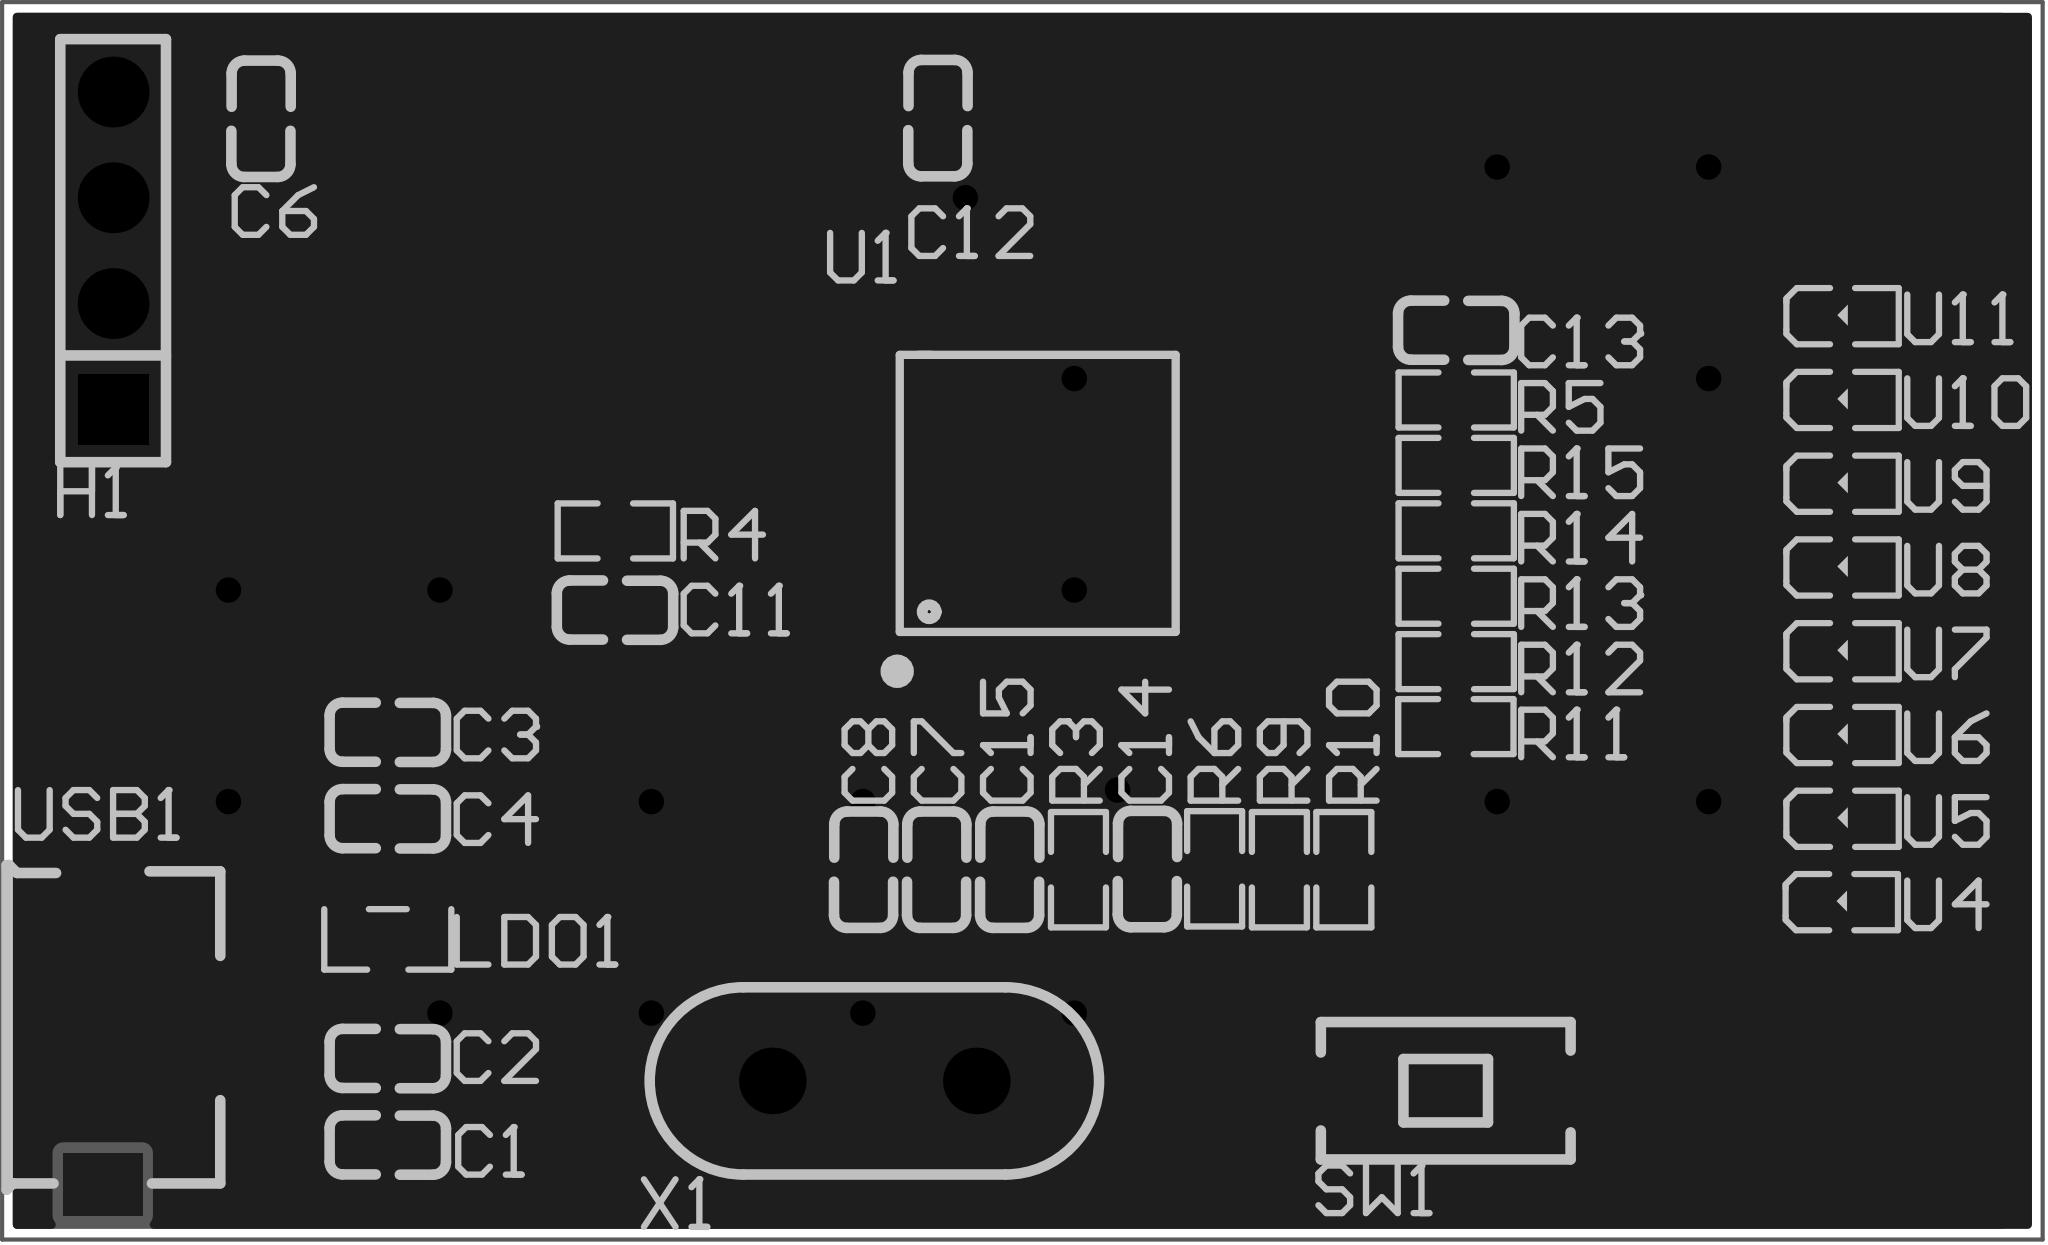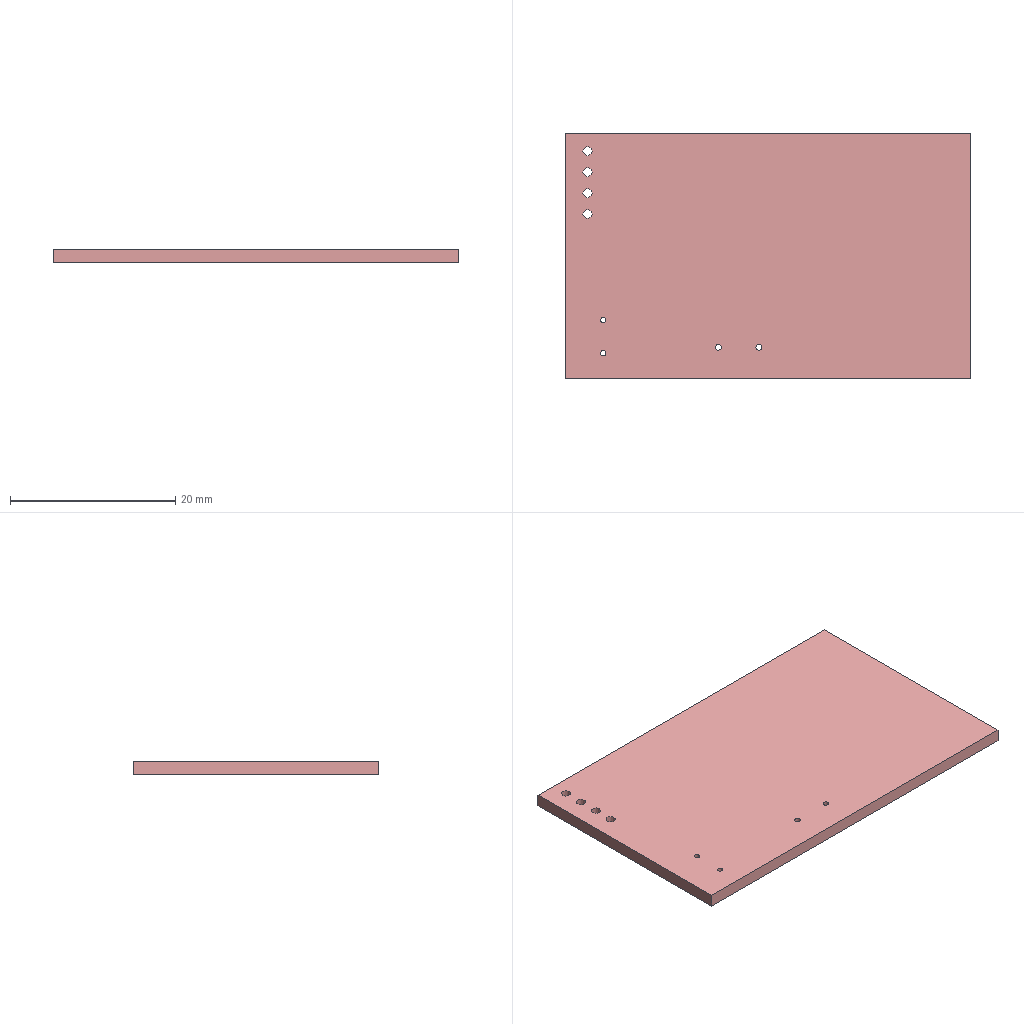Circuit board layout | Altium Designer | box 49 x 29.7 x 1.6 mm
Layer stack:
# Altium Designer layer stack of  (unit mm; dielectric type: 0 none, 1 core, 2 prepreg, 3 surface material)
index,name,kind,layer,copper_thickness_mm,dielectric_type,dielectric_thickness_mm,dielectric_material,dielectric_constant
0,Top Paste Mask Layer,other,,,,,,
1,Top Silkscreen Layer,other,,,,,,
2,Top Solder Mask Layer,dielectric,,,3,0.01,,3.3
3,Top Layer,copper,Top Layer,0.035,,,,
4,Dielectric1,dielectric,,,3,1.51,FR4,4.5
5,Bottom Layer,copper,Bottom Layer,0.035,,,,
6,Bottom Solder Mask Layer,dielectric,,,3,0.01,,3.3
7,Bottom Silkscreen Layer,other,,,,,,
8,Bottom Paste Mask Layer,other,,,,,,
# drill layer pairs: low layer,high layer
drill_pair,Top Layer,Bottom Layer
Part placement:
Designator,Comment,Layer,Footprint,Center-X(mm),Center-Y(mm),Rotation
R9,510Ω,TopLayer,R0603,111.584,88.892,90
R10,510Ω,TopLayer,R0603,113.133,88.892,90
R11,510Ω,TopLayer,R0603,115.824,92.329,180
R12,510Ω,TopLayer,R0603,115.833,93.889,180
R13,510Ω,TopLayer,R0603,115.833,95.46,180
R14,510Ω,TopLayer,R0603,115.833,97.031,180
R15,510Ω,TopLayer,R0603,115.833,98.602,180
U5,42-51/GHC-YW2X2K/3T,TopLayer,LED-SMD_L1.6-W0.8-FD_GREEN-1,125.114,90.14,180
U6,42-51/GHC-YW2X2K/3T,TopLayer,LED-SMD_L1.6-W0.8-FD_GREEN-1,125.114,92.152,180
U7,42-51/GHC-YW2X2K/3T,TopLayer,LED-SMD_L1.6-W0.8-FD_GREEN-1,125.114,94.163,180
U8,42-51/GHC-YW2X2K/3T,TopLayer,LED-SMD_L1.6-W0.8-FD_GREEN-1,125.114,96.175,180
U9,42-51/GHC-YW2X2K/3T,TopLayer,LED-SMD_L1.6-W0.8-FD_GREEN-1,125.114,98.187,180
U10,42-51/GHC-YW2X2K/3T,TopLayer,LED-SMD_L1.6-W0.8-FD_GREEN-1,125.114,100.199,180
U11,42-51/GHC-YW2X2K/3T,TopLayer,LED-SMD_L1.6-W0.8-FD_GREEN-1,125.114,102.211,180
C1,10uF,TopLayer,C0603,90.157,82.283,180
C2,100nF,TopLayer,C0603,90.157,84.359,180
C3,100nF,TopLayer,C0603,90.157,92.194,180
C4,10uF,TopLayer,C0603,90.157,90.118,180
C6,100nF,TopLayer,C0603,87.122,106.934,90
C7,20pF,TopLayer,C0603,103.354,88.9,90
C8,20pF,TopLayer,C0603,101.6,88.9,90
C11,100nF,TopLayer,C0603,95.631,95.123,0
C12,100nF,TopLayer,C0603,103.378,106.934,270
C13,100nF,TopLayer,C0603,115.825,101.85,180
C14,100nF,TopLayer,C0603,108.411,88.9,270
LDO1,SC662K-3.3V,TopLayer,SOT-23-3_L2.9-W1.3-P1.90-LS2.4-BR,90.165,87.219,90
R3,1kΩ,TopLayer,R0603,106.757,88.892,90
R4,10kΩ,TopLayer,R0603,95.631,97.028,0
R5,10kΩ,TopLayer,R0603,115.833,100.173,180
R6,510Ω,TopLayer,R0603,110.028,88.914,90
SW1,TS-1101-C-W,TopLayer,SW-SMD_L6.0-W3.3-LS8.0,115.443,83.566,180
U1,STM32F103C8T6,TopLayer,LQFP-48_L7.0-W7.0-P0.50-LS9.0-BL,105.791,97.917,0
U4,42-51/GHC-YW2X2K/3T,TopLayer,LED-SMD_L1.6-W0.8-FD_GREEN-1,125.095,88.138,180
USB1,920-D62A2021S10100,TopLayer,MICRO-USB-SMD_5P-P0.65-H-M_MICRO-USB-5P,84.709,85.09,270
X1,8MHz,TopLayer,OSC-TH_L10.0-W4.5-P5.00,101.854,83.82,90
C15,10uF,TopLayer,C0603,105.109,88.9,90
H1,,TopLayer,HDR-TH_4P-P2.54-V-M,83.566,103.759,90
Pad and via stacks:
# Altium Designer via and pad stacks of  (unit mm). Each distinct definition once, with the count of objects using it.
# via: kind,start_layer,end_layer,hole_mm,diameter_mm,mode(0 simple;1 top-mid-bottom;2 full stack),diameter_per_layer,count,example_net
# pad: kind,layer,hole_mm,hole_type(0 round;1 square;2 slot),plating,top_size,top_shape(1 round;2 rect;3 octagon;9 rounded rect),mid_size,bottom_size,mode,footprint,size_per_layer,count,example
pad,Top Layer,0,0,plated,0.8065x0.864,2,0.8065x0.864,0.8065x0.864,0,R0603,,22,R9.2
pad,Top Layer,0,0,plated,0.8x0.7,2,0.8x0.7,0.8x0.7,0,LED-SMD_L1.6-W0.8-FD_GREEN-1,,16,U5.1
pad,Top Layer,0,0,plated,0.8x0.9,2,0.8x0.9,0.8x0.9,0,C0603,,24,C1.2
pad,Top Layer,0,0,plated,1.25x0.7,2,1.25x0.7,1.25x0.7,0,SOT-23-3_L2.9-W1.3-P1.90-LS2.4-BR,,3,LDO1.1
pad,Top Layer,0,0,plated,1.9x1.5,2,1.9x1.5,1.9x1.5,0,SW-SMD_L6.0-W3.3-LS8.0,,2,SW1.1
pad,Top Layer,0,0,plated,0.27x1.5,1,0.27x1.5,0.27x1.5,0,LQFP-48_L7.0-W7.0-P0.50-LS9.0-BL,,24,U1.1
pad,Top Layer,0,0,plated,1.5x0.27,1,1.5x0.27,1.5x0.27,0,LQFP-48_L7.0-W7.0-P0.50-LS9.0-BL,,24,U1.13
pad,Top Layer,0,0,plated,1.35x0.4,2,1.35x0.4,1.35x0.4,0,MICRO-USB-SMD_5P-P0.65-H-M_MICRO-USB-5P,,5,USB1.5
pad,Top Layer,0,0,plated,1.5x1.9,2,1.5x1.9,1.5x1.9,0,MICRO-USB-SMD_5P-P0.65-H-M_MICRO-USB-5P,,2,USB1.0
pad,Top Layer,0,0,plated,1.9x1.9,2,1.9x1.9,1.9x1.9,0,MICRO-USB-SMD_5P-P0.65-H-M_MICRO-USB-5P,,2,USB1.0
pad,Multi-Layer,0.7,0,plated,1.6x1.6,1,1.6x1.6,1.6x1.6,0,OSC-TH_L10.0-W4.5-P5.00,,2,X1.2
pad,Multi-Layer,1.1,0,plated,1.7x1.7,2,1.7x1.7,1.7x1.7,0,HDR-TH_4P-P2.54-V-M,,1,H1.1
pad,Multi-Layer,1.1,0,plated,1.7x1.7,1,1.7x1.7,1.7x1.7,0,HDR-TH_4P-P2.54-V-M,,3,H1.2
via,Top Layer,Bottom Layer,0.3048,0.61,0,,18,DIO
Copper pours:
name,layer,net,type(0 solid;1 hatched;2 none)
Top Layer-GND,Top Layer,GND,0
Bottom Layer-GND,Bottom Layer,GND,0
Design rules, without the lines most boards share:
# Altium Designer design rules of  (exported by Altium Designer, unit mm)
# columns: name | kind | enabled | priority | scope1 | scope2 | descriptor | typed fields (field=value)
otherClearance | 52 | enabled | 1 | All | All | Hole To Hole Clearance (Gap=11.8mil) (All),(All) | gap=0.2997